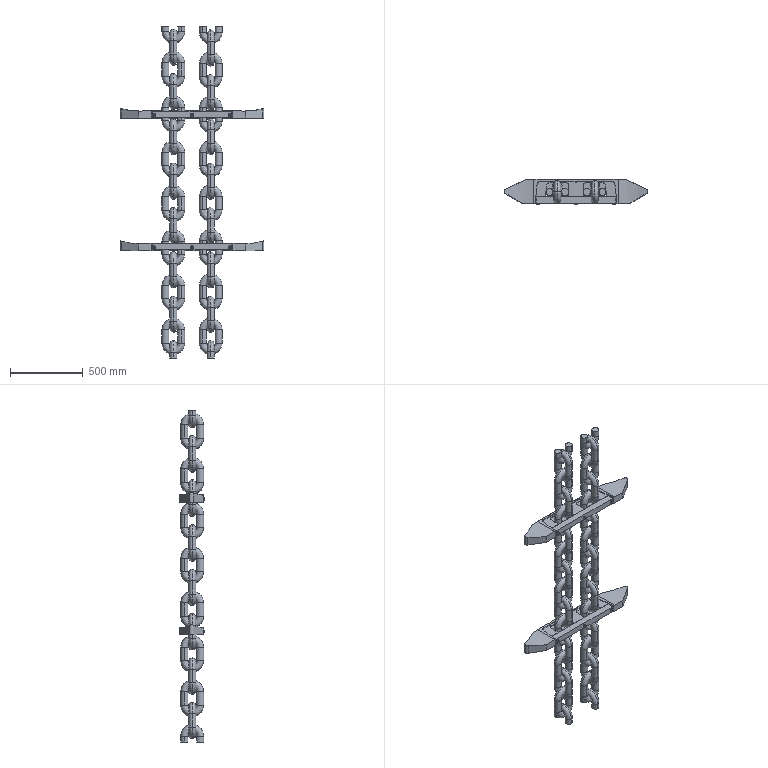Part | SolidWorks | features ReferencePattern 36, Cut 1, LocalChainPattern 1 | 48 solids | 916 faces | box 984.376 x 173.983 x 2274 mm | volume 39316055 mm3 | plane 300 | cylinder 224 | torus 204 | spline 116 | cone 72 | commonest cylinder face diameters 48 x132 10 x48 25 x12 33 x12 64 x8 33.92 x4